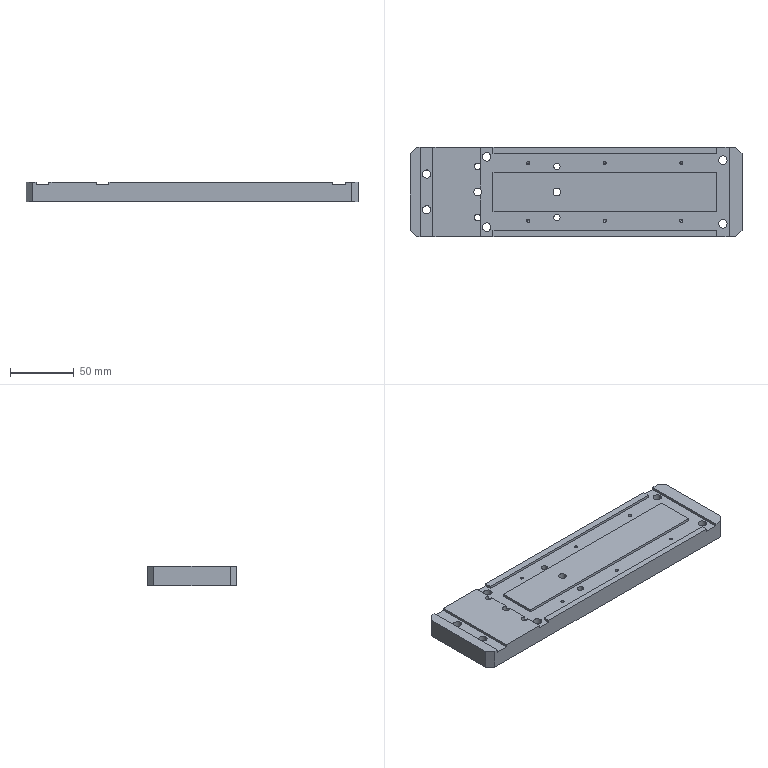Part | STEP file | PN_0024 | 1 solid | 94 faces | box 260 x 70 x 15 mm | volume 251185 mm3 | cylinder 44 | plane 38 | cone 12 | commonest cylinder face diameters 2.5 x12 5 x8 6.6 x8 11 x8 6 x4 6.5 x4